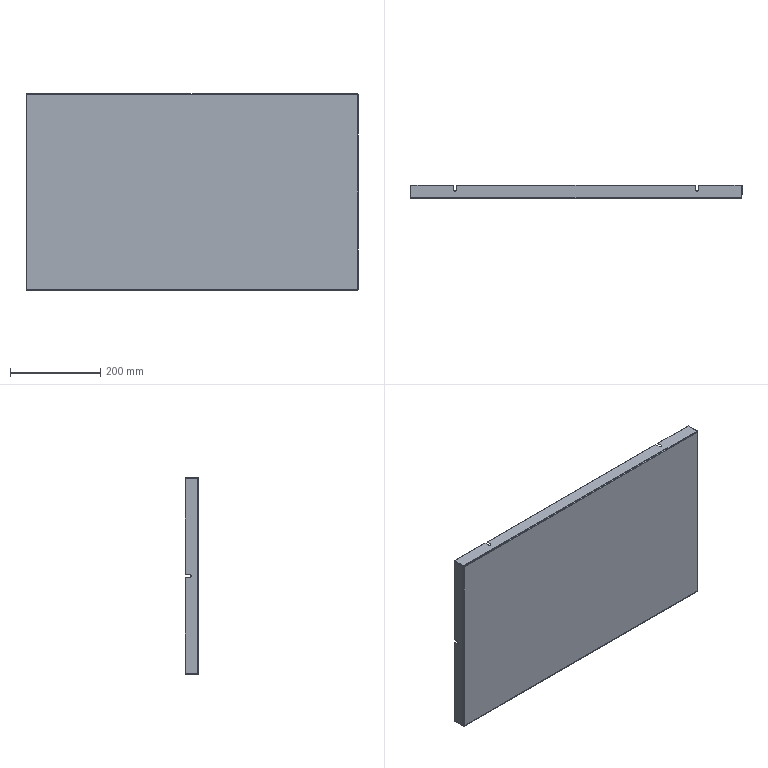Part | STEP file | JBJ-P-1000-09 | 1 solid | 62 faces | box 735 x 30 x 435 mm | volume 461490 mm3 | plane 40 | cylinder 14 | spline 8 | commonest cylinder face diameters 6.5 x6 2 x4 4.4 x4